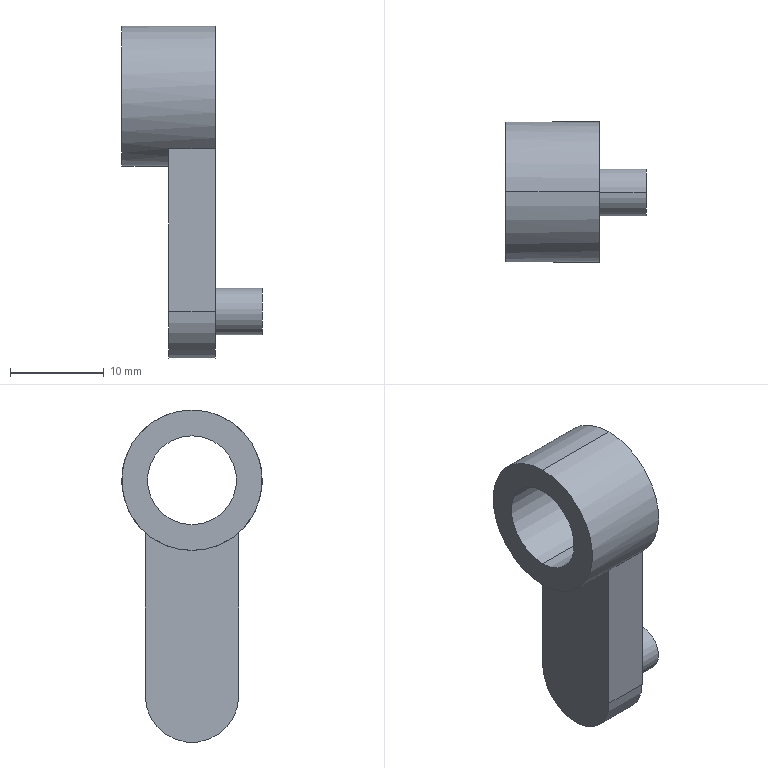Part | SolidWorks | 1 solid | 13 faces | box 15 x 15 x 35.5 mm | volume 2158 mm3 | cylinder 7 | plane 6 | commonest cylinder face diameters 5 x2 9.5 x2 15 x2 10 x1
STEP:
#1=CARTESIAN_POINT('',(-5.,0.,4.75));
#2=VERTEX_POINT('',#1);
#3=CARTESIAN_POINT('',(-5.,0.,-4.75));
#4=VERTEX_POINT('',#3);
#5=CARTESIAN_POINT('',(-5.,0.,0.));
#6=DIRECTION('',(1.,0.,0.));
#7=DIRECTION('',(0.,0.,-1.));
#8=AXIS2_PLACEMENT_3D('',#5,#6,#7);
#9=CIRCLE('',#8,4.75);
#10=EDGE_CURVE('',#2,#4,#9,.T.);
#11=ORIENTED_EDGE('',*,*,#10,.F.);
#12=CARTESIAN_POINT('',(5.,0.,4.75));
#13=VERTEX_POINT('',#12);
#14=CARTESIAN_POINT('',(-10.,0.,4.75));
#15=DIRECTION('',(1.,0.,0.));
#16=VECTOR('',#15,1000.);
#17=LINE('',#14,#16);
#18=EDGE_CURVE('',#2,#13,#17,.T.);
#19=ORIENTED_EDGE('',*,*,#18,.T.);
#20=CARTESIAN_POINT('',(5.,0.,-4.75));
#21=VERTEX_POINT('',#20);
#22=CARTESIAN_POINT('',(5.,0.,0.));
#23=DIRECTION('',(1.,0.,0.));
#24=DIRECTION('',(0.,0.,-1.));
#25=AXIS2_PLACEMENT_3D('',#22,#23,#24);
#26=CIRCLE('',#25,4.75);
#27=EDGE_CURVE('',#13,#21,#26,.T.);
#28=ORIENTED_EDGE('',*,*,#27,.T.);
#29=CARTESIAN_POINT('',(-10.,0.,-4.75));
#30=DIRECTION('',(1.,0.,0.));
#31=VECTOR('',#30,1000.);
#32=LINE('',#29,#31);
#33=EDGE_CURVE('',#4,#21,#32,.T.);
#34=ORIENTED_EDGE('',*,*,#33,.F.);
#35=EDGE_LOOP('',(#11,#19,#28,#34));
#36=FACE_OUTER_BOUND('',#35,.T.);
#37=CARTESIAN_POINT('',(-10.,0.,0.));
#38=DIRECTION('',(1.,0.,0.));
#39=DIRECTION('',(0.,0.,-1.));
#40=AXIS2_PLACEMENT_3D('',#37,#38,#39);
#41=CYLINDRICAL_SURFACE('',#40,4.75);
#42=ADVANCED_FACE('',(#36),#41,.F.);
#43=CARTESIAN_POINT('',(-5.,0.,-7.5));
#44=VERTEX_POINT('',#43);
#45=CARTESIAN_POINT('',(-5.,0.,7.5));
#46=VERTEX_POINT('',#45);
#47=CARTESIAN_POINT('',(-5.,0.,0.));
#48=DIRECTION('',(1.,0.,0.));
#49=DIRECTION('',(0.,0.,-1.));
#50=AXIS2_PLACEMENT_3D('',#47,#48,#49);
#51=CIRCLE('',#50,7.5);
#52=EDGE_CURVE('',#44,#46,#51,.T.);
#53=ORIENTED_EDGE('',*,*,#52,.T.);
#54=CARTESIAN_POINT('',(5.,0.,7.5));
#55=VERTEX_POINT('',#54);
#56=CARTESIAN_POINT('',(-5.,0.,7.5));
#57=DIRECTION('',(1.,0.,0.));
#58=VECTOR('',#57,1000.);
#59=LINE('',#56,#58);
#60=EDGE_CURVE('',#46,#55,#59,.T.);
#61=ORIENTED_EDGE('',*,*,#60,.T.);
#62=CARTESIAN_POINT('',(5.,5.,-5.59));
#63=VERTEX_POINT('',#62);
#64=CARTESIAN_POINT('',(5.,0.,0.));
#65=DIRECTION('',(1.,0.,0.));
#66=DIRECTION('',(0.,0.,-1.));
#67=AXIS2_PLACEMENT_3D('',#64,#65,#66);
#68=CIRCLE('',#67,7.5);
#69=EDGE_CURVE('',#63,#55,#68,.T.);
#70=ORIENTED_EDGE('',*,*,#69,.F.);
#71=CARTESIAN_POINT('',(0.,5.,-5.59));
#72=VERTEX_POINT('',#71);
#73=CARTESIAN_POINT('',(-5.,5.,-5.59));
#74=DIRECTION('',(1.,0.,0.));
#75=VECTOR('',#74,1000.);
#76=LINE('',#73,#75);
#77=EDGE_CURVE('',#72,#63,#76,.T.);
#78=ORIENTED_EDGE('',*,*,#77,.F.);
#79=CARTESIAN_POINT('',(0.,0.,-7.5));
#80=VERTEX_POINT('',#79);
#81=CARTESIAN_POINT('',(0.,0.,0.));
#82=DIRECTION('',(1.,0.,0.));
#83=DIRECTION('',(0.,0.,-1.));
#84=AXIS2_PLACEMENT_3D('',#81,#82,#83);
#85=CIRCLE('',#84,7.5);
#86=EDGE_CURVE('',#80,#72,#85,.T.);
#87=ORIENTED_EDGE('',*,*,#86,.F.);
#88=CARTESIAN_POINT('',(-5.,0.,-7.5));
#89=DIRECTION('',(1.,0.,0.));
#90=VECTOR('',#89,1000.);
#91=LINE('',#88,#90);
#92=EDGE_CURVE('',#44,#80,#91,.T.);
#93=ORIENTED_EDGE('',*,*,#92,.F.);
#94=EDGE_LOOP('',(#53,#61,#70,#78,#87,#93));
#95=FACE_OUTER_BOUND('',#94,.T.);
#96=CARTESIAN_POINT('',(-5.,0.,0.));
#97=DIRECTION('',(1.,0.,0.));
#98=DIRECTION('',(0.,0.,-1.));
#99=AXIS2_PLACEMENT_3D('',#96,#97,#98);
#100=CYLINDRICAL_SURFACE('',#99,7.5);
#101=ADVANCED_FACE('',(#95),#100,.T.);
#102=CARTESIAN_POINT('',(10.,0.,-25.5));
#103=VERTEX_POINT('',#102);
#104=CARTESIAN_POINT('',(10.,0.,-20.5));
#105=VERTEX_POINT('',#104);
#106=CARTESIAN_POINT('',(10.,0.,-23.));
#107=DIRECTION('',(1.,0.,0.));
#108=DIRECTION('',(0.,0.,-1.));
#109=AXIS2_PLACEMENT_3D('',#106,#107,#108);
#110=CIRCLE('',#109,2.5);
#111=EDGE_CURVE('',#103,#105,#110,.T.);
#112=ORIENTED_EDGE('',*,*,#111,.F.);
#113=CARTESIAN_POINT('',(5.,0.,-25.5));
#114=VERTEX_POINT('',#113);
#115=CARTESIAN_POINT('',(10.,0.,-25.5));
#116=DIRECTION('',(-1.,0.,0.));
#117=VECTOR('',#116,1000.);
#118=LINE('',#115,#117);
#119=EDGE_CURVE('',#103,#114,#118,.T.);
#120=ORIENTED_EDGE('',*,*,#119,.T.);
#121=CARTESIAN_POINT('',(5.,0.,-20.5));
#122=VERTEX_POINT('',#121);
#123=CARTESIAN_POINT('',(5.,0.,-23.));
#124=DIRECTION('',(1.,0.,0.));
#125=DIRECTION('',(0.,0.,-1.));
#126=AXIS2_PLACEMENT_3D('',#123,#124,#125);
#127=CIRCLE('',#126,2.5);
#128=EDGE_CURVE('',#114,#122,#127,.T.);
#129=ORIENTED_EDGE('',*,*,#128,.T.);
#130=CARTESIAN_POINT('',(10.,0.,-20.5));
#131=DIRECTION('',(-1.,0.,0.));
#132=VECTOR('',#131,1000.);
#133=LINE('',#130,#132);
#134=EDGE_CURVE('',#105,#122,#133,.T.);
#135=ORIENTED_EDGE('',*,*,#134,.F.);
#136=EDGE_LOOP('',(#112,#120,#129,#135));
#137=FACE_OUTER_BOUND('',#136,.T.);
#138=CARTESIAN_POINT('',(10.,0.,-23.));
#139=DIRECTION('',(-1.,0.,0.));
#140=DIRECTION('',(0.,0.,1.));
#141=AXIS2_PLACEMENT_3D('',#138,#139,#140);
#142=CYLINDRICAL_SURFACE('',#141,2.5);
#143=ADVANCED_FACE('',(#137),#142,.T.);
#144=CARTESIAN_POINT('',(5.,-5.,-5.59));
#145=VERTEX_POINT('',#144);
#146=CARTESIAN_POINT('',(5.,-5.,-23.));
#147=VERTEX_POINT('',#146);
#148=CARTESIAN_POINT('',(5.,-5.,0.));
#149=DIRECTION('',(0.,0.,-1.));
#150=VECTOR('',#149,1000.);
#151=LINE('',#148,#150);
#152=EDGE_CURVE('',#145,#147,#151,.T.);
#153=ORIENTED_EDGE('',*,*,#152,.F.);
#154=CARTESIAN_POINT('',(0.,-5.,-5.59));
#155=VERTEX_POINT('',#154);
#156=CARTESIAN_POINT('',(-5.,-5.,-5.59));
#157=DIRECTION('',(-1.,0.,0.));
#158=VECTOR('',#157,1000.);
#159=LINE('',#156,#158);
#160=EDGE_CURVE('',#145,#155,#159,.T.);
#161=ORIENTED_EDGE('',*,*,#160,.T.);
#162=CARTESIAN_POINT('',(0.,-5.,-23.));
#163=VERTEX_POINT('',#162);
#164=CARTESIAN_POINT('',(0.,-5.,0.));
#165=DIRECTION('',(0.,0.,-1.));
#166=VECTOR('',#165,1000.);
#167=LINE('',#164,#166);
#168=EDGE_CURVE('',#155,#163,#167,.T.);
#169=ORIENTED_EDGE('',*,*,#168,.T.);
#170=CARTESIAN_POINT('',(5.,-5.,-23.));
#171=DIRECTION('',(-1.,0.,0.));
#172=VECTOR('',#171,1000.);
#173=LINE('',#170,#172);
#174=EDGE_CURVE('',#147,#163,#173,.T.);
#175=ORIENTED_EDGE('',*,*,#174,.F.);
#176=EDGE_LOOP('',(#153,#161,#169,#175));
#177=FACE_OUTER_BOUND('',#176,.T.);
#178=CARTESIAN_POINT('',(5.,-5.,0.));
#179=DIRECTION('',(0.,1.,0.));
#180=DIRECTION('',(0.,0.,1.));
#181=AXIS2_PLACEMENT_3D('',#178,#179,#180);
#182=PLANE('',#181);
#183=ADVANCED_FACE('',(#177),#182,.F.);
#184=CARTESIAN_POINT('',(0.,5.,-23.));
#185=VERTEX_POINT('',#184);
#186=CARTESIAN_POINT('',(0.,0.,-23.));
#187=DIRECTION('',(1.,0.,0.));
#188=DIRECTION('',(0.,0.,-1.));
#189=AXIS2_PLACEMENT_3D('',#186,#187,#188);
#190=CIRCLE('',#189,5.);
#191=EDGE_CURVE('',#163,#185,#190,.T.);
#192=ORIENTED_EDGE('',*,*,#191,.T.);
#193=CARTESIAN_POINT('',(5.,5.,-23.));
#194=VERTEX_POINT('',#193);
#195=CARTESIAN_POINT('',(5.,5.,-23.));
#196=DIRECTION('',(-1.,0.,0.));
#197=VECTOR('',#196,1000.);
#198=LINE('',#195,#197);
#199=EDGE_CURVE('',#194,#185,#198,.T.);
#200=ORIENTED_EDGE('',*,*,#199,.F.);
#201=CARTESIAN_POINT('',(5.,0.,-23.));
#202=DIRECTION('',(1.,0.,0.));
#203=DIRECTION('',(0.,0.,-1.));
#204=AXIS2_PLACEMENT_3D('',#201,#202,#203);
#205=CIRCLE('',#204,5.);
#206=EDGE_CURVE('',#147,#194,#205,.T.);
#207=ORIENTED_EDGE('',*,*,#206,.F.);
#208=ORIENTED_EDGE('',*,*,#174,.T.);
#209=EDGE_LOOP('',(#192,#200,#207,#208));
#210=FACE_OUTER_BOUND('',#209,.T.);
#211=CARTESIAN_POINT('',(5.,0.,-23.));
#212=DIRECTION('',(-1.,0.,0.));
#213=DIRECTION('',(0.,0.,1.));
#214=AXIS2_PLACEMENT_3D('',#211,#212,#213);
#215=CYLINDRICAL_SURFACE('',#214,5.);
#216=ADVANCED_FACE('',(#210),#215,.T.);
#217=CARTESIAN_POINT('',(0.,5.,0.));
#218=DIRECTION('',(0.,0.,1.));
#219=VECTOR('',#218,1000.);
#220=LINE('',#217,#219);
#221=EDGE_CURVE('',#185,#72,#220,.T.);
#222=ORIENTED_EDGE('',*,*,#221,.T.);
#223=ORIENTED_EDGE('',*,*,#77,.T.);
#224=CARTESIAN_POINT('',(5.,5.,0.));
#225=DIRECTION('',(0.,0.,1.));
#226=VECTOR('',#225,1000.);
#227=LINE('',#224,#226);
#228=EDGE_CURVE('',#194,#63,#227,.T.);
#229=ORIENTED_EDGE('',*,*,#228,.F.);
#230=ORIENTED_EDGE('',*,*,#199,.T.);
#231=EDGE_LOOP('',(#222,#223,#229,#230));
#232=FACE_OUTER_BOUND('',#231,.T.);
#233=CARTESIAN_POINT('',(5.,5.,0.));
#234=DIRECTION('',(0.,-1.,0.));
#235=DIRECTION('',(0.,0.,-1.));
#236=AXIS2_PLACEMENT_3D('',#233,#234,#235);
#237=PLANE('',#236);
#238=ADVANCED_FACE('',(#232),#237,.F.);
#239=CARTESIAN_POINT('',(5.,0.,0.));
#240=DIRECTION('',(1.,0.,0.));
#241=DIRECTION('',(0.,0.,-1.));
#242=AXIS2_PLACEMENT_3D('',#239,#240,#241);
#243=CIRCLE('',#242,4.75);
#244=EDGE_CURVE('',#21,#13,#243,.T.);
#245=ORIENTED_EDGE('',*,*,#244,.F.);
#246=ORIENTED_EDGE('',*,*,#27,.F.);
#247=EDGE_LOOP('',(#245,#246));
#248=FACE_BOUND('',#247,.T.);
#249=ORIENTED_EDGE('',*,*,#69,.T.);
#250=CARTESIAN_POINT('',(5.,0.,0.));
#251=DIRECTION('',(1.,0.,0.));
#252=DIRECTION('',(0.,0.,-1.));
#253=AXIS2_PLACEMENT_3D('',#250,#251,#252);
#254=CIRCLE('',#253,7.5);
#255=EDGE_CURVE('',#55,#145,#254,.T.);
#256=ORIENTED_EDGE('',*,*,#255,.T.);
#257=ORIENTED_EDGE('',*,*,#152,.T.);
#258=ORIENTED_EDGE('',*,*,#206,.T.);
#259=ORIENTED_EDGE('',*,*,#228,.T.);
#260=EDGE_LOOP('',(#249,#256,#257,#258,#259));
#261=FACE_OUTER_BOUND('',#260,.T.);
#262=CARTESIAN_POINT('',(5.,0.,-23.));
#263=DIRECTION('',(1.,0.,0.));
#264=DIRECTION('',(0.,0.,-1.));
#265=AXIS2_PLACEMENT_3D('',#262,#263,#264);
#266=CIRCLE('',#265,2.5);
#267=EDGE_CURVE('',#122,#114,#266,.T.);
#268=ORIENTED_EDGE('',*,*,#267,.F.);
#269=ORIENTED_EDGE('',*,*,#128,.F.);
#270=EDGE_LOOP('',(#268,#269));
#271=FACE_BOUND('',#270,.T.);
#272=CARTESIAN_POINT('',(5.,0.,0.));
#273=DIRECTION('',(1.,0.,0.));
#274=DIRECTION('',(0.,0.,-1.));
#275=AXIS2_PLACEMENT_3D('',#272,#273,#274);
#276=PLANE('',#275);
#277=ADVANCED_FACE('',(#248,#261,#271),#276,.T.);
#278=ORIENTED_EDGE('',*,*,#168,.F.);
#279=CARTESIAN_POINT('',(0.,0.,0.));
#280=DIRECTION('',(1.,0.,0.));
#281=DIRECTION('',(0.,0.,-1.));
#282=AXIS2_PLACEMENT_3D('',#279,#280,#281);
#283=CIRCLE('',#282,7.5);
#284=EDGE_CURVE('',#155,#80,#283,.T.);
#285=ORIENTED_EDGE('',*,*,#284,.T.);
#286=ORIENTED_EDGE('',*,*,#86,.T.);
#287=ORIENTED_EDGE('',*,*,#221,.F.);
#288=ORIENTED_EDGE('',*,*,#191,.F.);
#289=EDGE_LOOP('',(#278,#285,#286,#287,#288));
#290=FACE_OUTER_BOUND('',#289,.T.);
#291=CARTESIAN_POINT('',(0.,0.,0.));
#292=DIRECTION('',(1.,0.,0.));
#293=DIRECTION('',(0.,0.,-1.));
#294=AXIS2_PLACEMENT_3D('',#291,#292,#293);
#295=PLANE('',#294);
#296=ADVANCED_FACE('',(#290),#295,.F.);
#297=ORIENTED_EDGE('',*,*,#119,.F.);
#298=CARTESIAN_POINT('',(10.,0.,-23.));
#299=DIRECTION('',(1.,0.,0.));
#300=DIRECTION('',(0.,0.,-1.));
#301=AXIS2_PLACEMENT_3D('',#298,#299,#300);
#302=CIRCLE('',#301,2.5);
#303=EDGE_CURVE('',#105,#103,#302,.T.);
#304=ORIENTED_EDGE('',*,*,#303,.F.);
#305=ORIENTED_EDGE('',*,*,#134,.T.);
#306=ORIENTED_EDGE('',*,*,#267,.T.);
#307=EDGE_LOOP('',(#297,#304,#305,#306));
#308=FACE_OUTER_BOUND('',#307,.T.);
#309=CARTESIAN_POINT('',(10.,0.,-23.));
#310=DIRECTION('',(-1.,0.,0.));
#311=DIRECTION('',(0.,0.,1.));
#312=AXIS2_PLACEMENT_3D('',#309,#310,#311);
#313=CYLINDRICAL_SURFACE('',#312,2.5);
#314=ADVANCED_FACE('',(#308),#313,.T.);
#315=ORIENTED_EDGE('',*,*,#303,.T.);
#316=ORIENTED_EDGE('',*,*,#111,.T.);
#317=EDGE_LOOP('',(#315,#316));
#318=FACE_OUTER_BOUND('',#317,.T.);
#319=CARTESIAN_POINT('',(10.,0.,-23.));
#320=DIRECTION('',(1.,0.,0.));
#321=DIRECTION('',(0.,0.,-1.));
#322=AXIS2_PLACEMENT_3D('',#319,#320,#321);
#323=PLANE('',#322);
#324=ADVANCED_FACE('',(#318),#323,.T.);
#325=ORIENTED_EDGE('',*,*,#60,.F.);
#326=CARTESIAN_POINT('',(-5.,0.,0.));
#327=DIRECTION('',(1.,0.,0.));
#328=DIRECTION('',(0.,0.,-1.));
#329=AXIS2_PLACEMENT_3D('',#326,#327,#328);
#330=CIRCLE('',#329,7.5);
#331=EDGE_CURVE('',#46,#44,#330,.T.);
#332=ORIENTED_EDGE('',*,*,#331,.T.);
#333=ORIENTED_EDGE('',*,*,#92,.T.);
#334=ORIENTED_EDGE('',*,*,#284,.F.);
#335=ORIENTED_EDGE('',*,*,#160,.F.);
#336=ORIENTED_EDGE('',*,*,#255,.F.);
#337=EDGE_LOOP('',(#325,#332,#333,#334,#335,#336));
#338=FACE_OUTER_BOUND('',#337,.T.);
#339=CARTESIAN_POINT('',(-5.,0.,0.));
#340=DIRECTION('',(1.,0.,0.));
#341=DIRECTION('',(0.,0.,-1.));
#342=AXIS2_PLACEMENT_3D('',#339,#340,#341);
#343=CYLINDRICAL_SURFACE('',#342,7.5);
#344=ADVANCED_FACE('',(#338),#343,.T.);
#345=CARTESIAN_POINT('',(-5.,0.,0.));
#346=DIRECTION('',(1.,0.,0.));
#347=DIRECTION('',(0.,0.,-1.));
#348=AXIS2_PLACEMENT_3D('',#345,#346,#347);
#349=CIRCLE('',#348,4.75);
#350=EDGE_CURVE('',#4,#2,#349,.T.);
#351=ORIENTED_EDGE('',*,*,#350,.T.);
#352=ORIENTED_EDGE('',*,*,#10,.T.);
#353=EDGE_LOOP('',(#351,#352));
#354=FACE_BOUND('',#353,.T.);
#355=ORIENTED_EDGE('',*,*,#52,.F.);
#356=ORIENTED_EDGE('',*,*,#331,.F.);
#357=EDGE_LOOP('',(#355,#356));
#358=FACE_OUTER_BOUND('',#357,.T.);
#359=CARTESIAN_POINT('',(-5.,0.,0.));
#360=DIRECTION('',(1.,0.,0.));
#361=DIRECTION('',(0.,0.,-1.));
#362=AXIS2_PLACEMENT_3D('',#359,#360,#361);
#363=PLANE('',#362);
#364=ADVANCED_FACE('',(#354,#358),#363,.F.);
#365=ORIENTED_EDGE('',*,*,#18,.F.);
#366=ORIENTED_EDGE('',*,*,#350,.F.);
#367=ORIENTED_EDGE('',*,*,#33,.T.);
#368=ORIENTED_EDGE('',*,*,#244,.T.);
#369=EDGE_LOOP('',(#365,#366,#367,#368));
#370=FACE_OUTER_BOUND('',#369,.T.);
#371=CARTESIAN_POINT('',(-10.,0.,0.));
#372=DIRECTION('',(1.,0.,0.));
#373=DIRECTION('',(0.,0.,-1.));
#374=AXIS2_PLACEMENT_3D('',#371,#372,#373);
#375=CYLINDRICAL_SURFACE('',#374,4.75);
#376=ADVANCED_FACE('',(#370),#375,.F.);
#377=CLOSED_SHELL('',(#42,#101,#143,#183,#216,#238,#277,#296,#314,#324,#344,#364,#376));
#378=MANIFOLD_SOLID_BREP('',#377);
#379=CARTESIAN_POINT('',(0.,0.,0.));
#380=DIRECTION('',(0.,0.,1.));
#381=DIRECTION('',(1.,0.,0.));
#382=AXIS2_PLACEMENT_3D('',#379,#380,#381);
#383=(LENGTH_UNIT()NAMED_UNIT(*)SI_UNIT(.MILLI.,.METRE.));
#384=UNCERTAINTY_MEASURE_WITH_UNIT(LENGTH_MEASURE(0.00001),#383,'','');
#385=(NAMED_UNIT(*)PLANE_ANGLE_UNIT()SI_UNIT($,.RADIAN.));
#386=(NAMED_UNIT(*)SI_UNIT($,.STERADIAN.)SOLID_ANGLE_UNIT());
#387=(GEOMETRIC_REPRESENTATION_CONTEXT(3)GLOBAL_UNCERTAINTY_ASSIGNED_CONTEXT((#384))GLOBAL_UNIT_ASSIGNED_CONTEXT((#383,#385,#386))REPRESENTATION_CONTEXT('',''));
#388=ADVANCED_BREP_SHAPE_REPRESENTATION('',(#378,#382),#387);